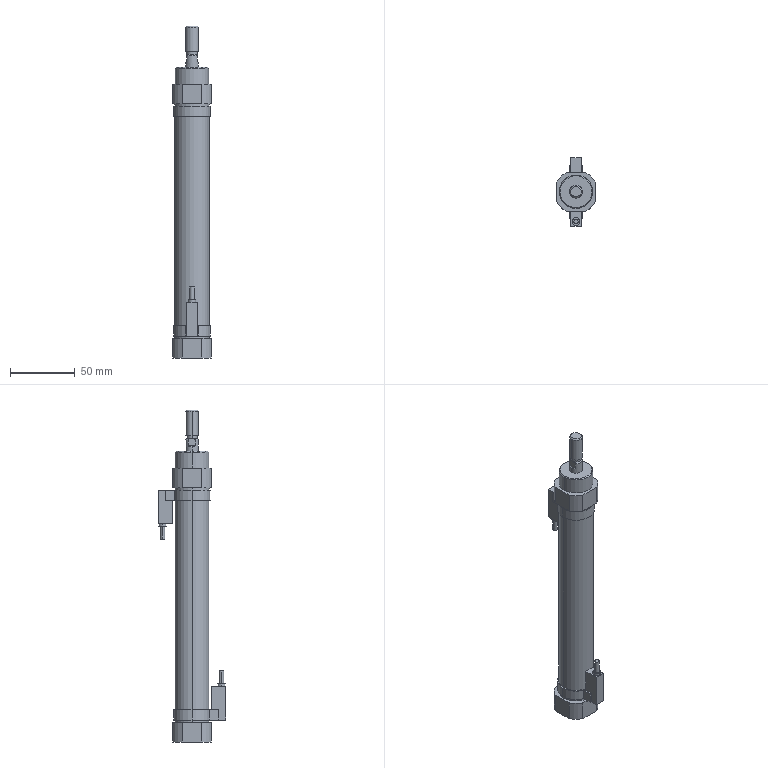Part | STEP file | Bag feed cylinder CDM2BZ25-150-C73 (0) | 1 solid | 106 faces | box 30 x 52.6 x 257 mm | volume 140263 mm3 | plane 54 | cylinder 42 | cone 10 | commonest cylinder face diameters 28.6 x8 33.5 x8 26.6 x6 3.4 x4 6 x4 8.57 x4